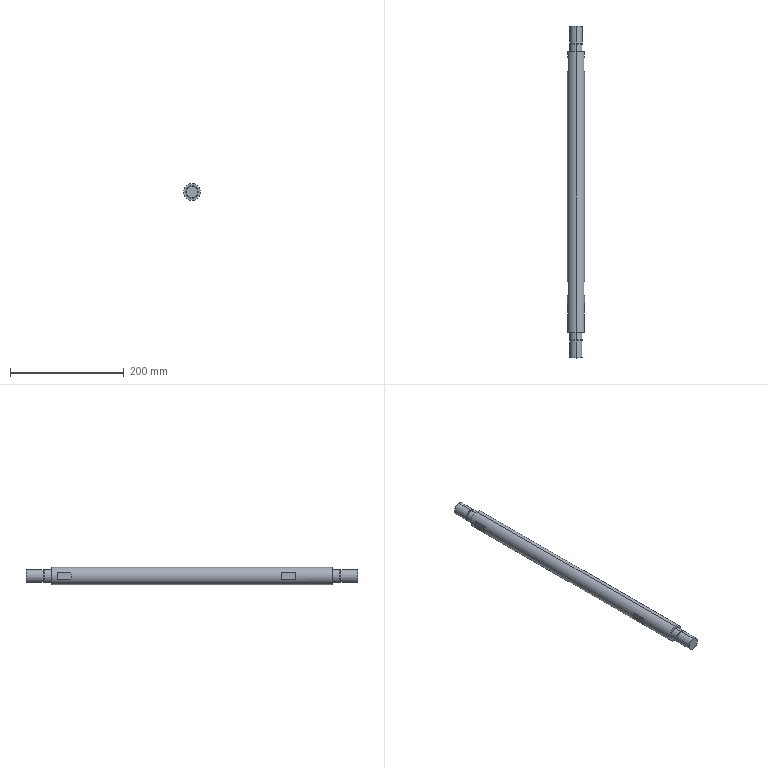Part | SolidWorks | features BaseBody 1 | 1 solid | 38 faces | box 30 x 585 x 30 mm | volume 382505 mm3 | plane 20 | cylinder 14 | cone 4 | commonest cylinder face diameters 22 x8 20 x4 30 x2
STEP:
#1=CARTESIAN_POINT('',(0.,30.,-11.));
#2=VERTEX_POINT('',#1);
#3=CARTESIAN_POINT('',(0.,30.,11.));
#4=VERTEX_POINT('',#3);
#5=CARTESIAN_POINT('',(0.,30.,0.));
#6=DIRECTION('',(0.,-1.,0.));
#7=DIRECTION('',(0.,0.,-1.));
#8=AXIS2_PLACEMENT_3D('',#5,#6,#7);
#9=CIRCLE('',#8,11.);
#10=EDGE_CURVE('',#2,#4,#9,.T.);
#11=ORIENTED_EDGE('',*,*,#10,.T.);
#12=CARTESIAN_POINT('',(0.,0.5,11.));
#13=VERTEX_POINT('',#12);
#14=CARTESIAN_POINT('',(0.,45.,11.));
#15=DIRECTION('',(0.,-1.,0.));
#16=VECTOR('',#15,1000.);
#17=LINE('',#14,#16);
#18=EDGE_CURVE('',#4,#13,#17,.T.);
#19=ORIENTED_EDGE('',*,*,#18,.T.);
#20=CARTESIAN_POINT('',(0.,0.5,-11.));
#21=VERTEX_POINT('',#20);
#22=CARTESIAN_POINT('',(0.,0.5,0.));
#23=DIRECTION('',(0.,1.,0.));
#24=DIRECTION('',(0.,0.,1.));
#25=AXIS2_PLACEMENT_3D('',#22,#23,#24);
#26=CIRCLE('',#25,11.);
#27=EDGE_CURVE('',#13,#21,#26,.T.);
#28=ORIENTED_EDGE('',*,*,#27,.T.);
#29=CARTESIAN_POINT('',(0.,45.,-11.));
#30=DIRECTION('',(0.,-1.,0.));
#31=VECTOR('',#30,1000.);
#32=LINE('',#29,#31);
#33=EDGE_CURVE('',#2,#21,#32,.T.);
#34=ORIENTED_EDGE('',*,*,#33,.F.);
#35=EDGE_LOOP('',(#11,#19,#28,#34));
#36=FACE_OUTER_BOUND('',#35,.T.);
#37=CARTESIAN_POINT('',(0.,45.,0.));
#38=DIRECTION('',(0.,-1.,0.));
#39=DIRECTION('',(0.,0.,-1.));
#40=AXIS2_PLACEMENT_3D('',#37,#38,#39);
#41=CYLINDRICAL_SURFACE('',#40,11.);
#42=ADVANCED_FACE('',(#36),#41,.T.);
#43=CARTESIAN_POINT('',(0.,0.,-10.5));
#44=VERTEX_POINT('',#43);
#45=CARTESIAN_POINT('',(0.,0.,10.5));
#46=VERTEX_POINT('',#45);
#47=CARTESIAN_POINT('',(0.,0.,0.));
#48=DIRECTION('',(0.,-1.,0.));
#49=DIRECTION('',(0.,0.,1.));
#50=AXIS2_PLACEMENT_3D('',#47,#48,#49);
#51=CIRCLE('',#50,10.5);
#52=EDGE_CURVE('',#44,#46,#51,.T.);
#53=ORIENTED_EDGE('',*,*,#52,.F.);
#54=CARTESIAN_POINT('',(0.,0.,-10.5));
#55=DIRECTION('',(0.,0.7071,-0.7071));
#56=VECTOR('',#55,1000.);
#57=LINE('',#54,#56);
#58=EDGE_CURVE('',#44,#21,#57,.T.);
#59=ORIENTED_EDGE('',*,*,#58,.T.);
#60=ORIENTED_EDGE('',*,*,#27,.F.);
#61=CARTESIAN_POINT('',(0.,0.,10.5));
#62=DIRECTION('',(0.,0.7071,0.7071));
#63=VECTOR('',#62,1000.);
#64=LINE('',#61,#63);
#65=EDGE_CURVE('',#46,#13,#64,.T.);
#66=ORIENTED_EDGE('',*,*,#65,.F.);
#67=EDGE_LOOP('',(#53,#59,#60,#66));
#68=FACE_OUTER_BOUND('',#67,.T.);
#69=CARTESIAN_POINT('',(0.,0.,0.));
#70=DIRECTION('',(0.,1.,0.));
#71=DIRECTION('',(0.,0.,1.));
#72=AXIS2_PLACEMENT_3D('',#69,#70,#71);
#73=CONICAL_SURFACE('',#72,10.5,0.7854);
#74=ADVANCED_FACE('',(#68),#73,.T.);
#75=CARTESIAN_POINT('',(0.,32.,-10.));
#76=VERTEX_POINT('',#75);
#77=CARTESIAN_POINT('',(0.,32.,10.));
#78=VERTEX_POINT('',#77);
#79=CARTESIAN_POINT('',(0.,32.,0.));
#80=DIRECTION('',(0.,-1.,0.));
#81=DIRECTION('',(0.,0.,-1.));
#82=AXIS2_PLACEMENT_3D('',#79,#80,#81);
#83=CIRCLE('',#82,10.);
#84=EDGE_CURVE('',#76,#78,#83,.T.);
#85=ORIENTED_EDGE('',*,*,#84,.T.);
#86=CARTESIAN_POINT('',(0.,30.,10.));
#87=VERTEX_POINT('',#86);
#88=CARTESIAN_POINT('',(0.,0.,10.));
#89=DIRECTION('',(0.,-1.,0.));
#90=VECTOR('',#89,1000.);
#91=LINE('',#88,#90);
#92=EDGE_CURVE('',#78,#87,#91,.T.);
#93=ORIENTED_EDGE('',*,*,#92,.T.);
#94=CARTESIAN_POINT('',(0.,30.,-10.));
#95=VERTEX_POINT('',#94);
#96=CARTESIAN_POINT('',(0.,30.,0.));
#97=DIRECTION('',(0.,-1.,0.));
#98=DIRECTION('',(0.,0.,-1.));
#99=AXIS2_PLACEMENT_3D('',#96,#97,#98);
#100=CIRCLE('',#99,10.);
#101=EDGE_CURVE('',#95,#87,#100,.T.);
#102=ORIENTED_EDGE('',*,*,#101,.F.);
#103=CARTESIAN_POINT('',(0.,0.,-10.));
#104=DIRECTION('',(0.,-1.,0.));
#105=VECTOR('',#104,1000.);
#106=LINE('',#103,#105);
#107=EDGE_CURVE('',#76,#95,#106,.T.);
#108=ORIENTED_EDGE('',*,*,#107,.F.);
#109=EDGE_LOOP('',(#85,#93,#102,#108));
#110=FACE_OUTER_BOUND('',#109,.T.);
#111=CARTESIAN_POINT('',(0.,0.,0.));
#112=DIRECTION('',(0.,-1.,0.));
#113=DIRECTION('',(0.,0.,-1.));
#114=AXIS2_PLACEMENT_3D('',#111,#112,#113);
#115=CYLINDRICAL_SURFACE('',#114,10.);
#116=ADVANCED_FACE('',(#110),#115,.T.);
#117=CARTESIAN_POINT('',(0.,45.,-11.));
#118=VERTEX_POINT('',#117);
#119=CARTESIAN_POINT('',(0.,45.,11.));
#120=VERTEX_POINT('',#119);
#121=CARTESIAN_POINT('',(0.,45.,0.));
#122=DIRECTION('',(0.,-1.,0.));
#123=DIRECTION('',(0.,0.,-1.));
#124=AXIS2_PLACEMENT_3D('',#121,#122,#123);
#125=CIRCLE('',#124,11.);
#126=EDGE_CURVE('',#118,#120,#125,.T.);
#127=ORIENTED_EDGE('',*,*,#126,.T.);
#128=CARTESIAN_POINT('',(0.,32.,11.));
#129=VERTEX_POINT('',#128);
#130=CARTESIAN_POINT('',(0.,45.,11.));
#131=DIRECTION('',(0.,-1.,0.));
#132=VECTOR('',#131,1000.);
#133=LINE('',#130,#132);
#134=EDGE_CURVE('',#120,#129,#133,.T.);
#135=ORIENTED_EDGE('',*,*,#134,.T.);
#136=CARTESIAN_POINT('',(0.,32.,-11.));
#137=VERTEX_POINT('',#136);
#138=CARTESIAN_POINT('',(0.,32.,0.));
#139=DIRECTION('',(0.,-1.,0.));
#140=DIRECTION('',(0.,0.,-1.));
#141=AXIS2_PLACEMENT_3D('',#138,#139,#140);
#142=CIRCLE('',#141,11.);
#143=EDGE_CURVE('',#137,#129,#142,.T.);
#144=ORIENTED_EDGE('',*,*,#143,.F.);
#145=CARTESIAN_POINT('',(0.,45.,-11.));
#146=DIRECTION('',(0.,-1.,0.));
#147=VECTOR('',#146,1000.);
#148=LINE('',#145,#147);
#149=EDGE_CURVE('',#118,#137,#148,.T.);
#150=ORIENTED_EDGE('',*,*,#149,.F.);
#151=EDGE_LOOP('',(#127,#135,#144,#150));
#152=FACE_OUTER_BOUND('',#151,.T.);
#153=CARTESIAN_POINT('',(0.,45.,0.));
#154=DIRECTION('',(0.,-1.,0.));
#155=DIRECTION('',(0.,0.,-1.));
#156=AXIS2_PLACEMENT_3D('',#153,#154,#155);
#157=CYLINDRICAL_SURFACE('',#156,11.);
#158=ADVANCED_FACE('',(#152),#157,.T.);
#159=CARTESIAN_POINT('',(13.5,505.,6.538));
#160=VERTEX_POINT('',#159);
#161=CARTESIAN_POINT('',(13.5,530.,6.538));
#162=VERTEX_POINT('',#161);
#163=CARTESIAN_POINT('',(13.5,585.,6.538));
#164=DIRECTION('',(0.,1.,0.));
#165=VECTOR('',#164,1000.);
#166=LINE('',#163,#165);
#167=EDGE_CURVE('',#160,#162,#166,.T.);
#168=ORIENTED_EDGE('',*,*,#167,.T.);
#169=CARTESIAN_POINT('',(13.5,530.,-6.538));
#170=VERTEX_POINT('',#169);
#171=CARTESIAN_POINT('',(0.,530.,0.));
#172=DIRECTION('',(0.,1.,0.));
#173=DIRECTION('',(0.,0.,1.));
#174=AXIS2_PLACEMENT_3D('',#171,#172,#173);
#175=CIRCLE('',#174,15.);
#176=EDGE_CURVE('',#162,#170,#175,.T.);
#177=ORIENTED_EDGE('',*,*,#176,.T.);
#178=CARTESIAN_POINT('',(13.5,505.,-6.538));
#179=VERTEX_POINT('',#178);
#180=CARTESIAN_POINT('',(13.5,585.,-6.538));
#181=DIRECTION('',(0.,-1.,0.));
#182=VECTOR('',#181,1000.);
#183=LINE('',#180,#182);
#184=EDGE_CURVE('',#170,#179,#183,.T.);
#185=ORIENTED_EDGE('',*,*,#184,.T.);
#186=CARTESIAN_POINT('',(0.,505.,0.));
#187=DIRECTION('',(0.,-1.,0.));
#188=DIRECTION('',(0.,0.,-1.));
#189=AXIS2_PLACEMENT_3D('',#186,#187,#188);
#190=CIRCLE('',#189,15.);
#191=EDGE_CURVE('',#179,#160,#190,.T.);
#192=ORIENTED_EDGE('',*,*,#191,.T.);
#193=EDGE_LOOP('',(#168,#177,#185,#192));
#194=FACE_BOUND('',#193,.T.);
#195=CARTESIAN_POINT('',(13.5,135.,-6.538));
#196=VERTEX_POINT('',#195);
#197=CARTESIAN_POINT('',(13.5,110.,-6.538));
#198=VERTEX_POINT('',#197);
#199=CARTESIAN_POINT('',(13.5,585.,-6.538));
#200=DIRECTION('',(0.,-1.,0.));
#201=VECTOR('',#200,1000.);
#202=LINE('',#199,#201);
#203=EDGE_CURVE('',#196,#198,#202,.T.);
#204=ORIENTED_EDGE('',*,*,#203,.T.);
#205=CARTESIAN_POINT('',(13.5,110.,6.538));
#206=VERTEX_POINT('',#205);
#207=CARTESIAN_POINT('',(0.,110.,0.));
#208=DIRECTION('',(0.,-1.,0.));
#209=DIRECTION('',(0.,0.,-1.));
#210=AXIS2_PLACEMENT_3D('',#207,#208,#209);
#211=CIRCLE('',#210,15.);
#212=EDGE_CURVE('',#198,#206,#211,.T.);
#213=ORIENTED_EDGE('',*,*,#212,.T.);
#214=CARTESIAN_POINT('',(13.5,135.,6.538));
#215=VERTEX_POINT('',#214);
#216=CARTESIAN_POINT('',(13.5,585.,6.538));
#217=DIRECTION('',(0.,1.,0.));
#218=VECTOR('',#217,1000.);
#219=LINE('',#216,#218);
#220=EDGE_CURVE('',#206,#215,#219,.T.);
#221=ORIENTED_EDGE('',*,*,#220,.T.);
#222=CARTESIAN_POINT('',(0.,135.,0.));
#223=DIRECTION('',(0.,1.,0.));
#224=DIRECTION('',(0.,0.,1.));
#225=AXIS2_PLACEMENT_3D('',#222,#223,#224);
#226=CIRCLE('',#225,15.);
#227=EDGE_CURVE('',#215,#196,#226,.T.);
#228=ORIENTED_EDGE('',*,*,#227,.T.);
#229=EDGE_LOOP('',(#204,#213,#221,#228));
#230=FACE_BOUND('',#229,.T.);
#231=CARTESIAN_POINT('',(0.,540.,15.));
#232=VERTEX_POINT('',#231);
#233=CARTESIAN_POINT('',(0.,540.,-15.));
#234=VERTEX_POINT('',#233);
#235=CARTESIAN_POINT('',(0.,540.,0.));
#236=DIRECTION('',(0.,1.,0.));
#237=DIRECTION('',(0.,0.,1.));
#238=AXIS2_PLACEMENT_3D('',#235,#236,#237);
#239=CIRCLE('',#238,15.);
#240=EDGE_CURVE('',#232,#234,#239,.T.);
#241=ORIENTED_EDGE('',*,*,#240,.F.);
#242=CARTESIAN_POINT('',(0.,45.,15.));
#243=VERTEX_POINT('',#242);
#244=CARTESIAN_POINT('',(0.,585.,15.));
#245=DIRECTION('',(0.,-1.,0.));
#246=VECTOR('',#245,1000.);
#247=LINE('',#244,#246);
#248=EDGE_CURVE('',#232,#243,#247,.T.);
#249=ORIENTED_EDGE('',*,*,#248,.T.);
#250=CARTESIAN_POINT('',(0.,45.,-15.));
#251=VERTEX_POINT('',#250);
#252=CARTESIAN_POINT('',(0.,45.,0.));
#253=DIRECTION('',(0.,-1.,0.));
#254=DIRECTION('',(0.,0.,-1.));
#255=AXIS2_PLACEMENT_3D('',#252,#253,#254);
#256=CIRCLE('',#255,15.);
#257=EDGE_CURVE('',#251,#243,#256,.T.);
#258=ORIENTED_EDGE('',*,*,#257,.F.);
#259=CARTESIAN_POINT('',(0.,585.,-15.));
#260=DIRECTION('',(0.,-1.,0.));
#261=VECTOR('',#260,1000.);
#262=LINE('',#259,#261);
#263=EDGE_CURVE('',#234,#251,#262,.T.);
#264=ORIENTED_EDGE('',*,*,#263,.F.);
#265=EDGE_LOOP('',(#241,#249,#258,#264));
#266=FACE_OUTER_BOUND('',#265,.T.);
#267=CARTESIAN_POINT('',(0.,585.,0.));
#268=DIRECTION('',(0.,-1.,0.));
#269=DIRECTION('',(0.,0.,-1.));
#270=AXIS2_PLACEMENT_3D('',#267,#268,#269);
#271=CYLINDRICAL_SURFACE('',#270,15.);
#272=ADVANCED_FACE('',(#194,#230,#266),#271,.T.);
#273=CARTESIAN_POINT('',(0.,540.,11.));
#274=VERTEX_POINT('',#273);
#275=CARTESIAN_POINT('',(0.,540.,-11.));
#276=VERTEX_POINT('',#275);
#277=CARTESIAN_POINT('',(0.,540.,0.));
#278=DIRECTION('',(0.,1.,0.));
#279=DIRECTION('',(0.,0.,1.));
#280=AXIS2_PLACEMENT_3D('',#277,#278,#279);
#281=CIRCLE('',#280,11.);
#282=EDGE_CURVE('',#274,#276,#281,.T.);
#283=ORIENTED_EDGE('',*,*,#282,.T.);
#284=CARTESIAN_POINT('',(0.,553.,-11.));
#285=VERTEX_POINT('',#284);
#286=CARTESIAN_POINT('',(0.,540.,-11.));
#287=DIRECTION('',(0.,1.,0.));
#288=VECTOR('',#287,1000.);
#289=LINE('',#286,#288);
#290=EDGE_CURVE('',#276,#285,#289,.T.);
#291=ORIENTED_EDGE('',*,*,#290,.T.);
#292=CARTESIAN_POINT('',(0.,553.,11.));
#293=VERTEX_POINT('',#292);
#294=CARTESIAN_POINT('',(0.,553.,0.));
#295=DIRECTION('',(0.,-1.,0.));
#296=DIRECTION('',(0.,0.,-1.));
#297=AXIS2_PLACEMENT_3D('',#294,#295,#296);
#298=CIRCLE('',#297,11.);
#299=EDGE_CURVE('',#285,#293,#298,.T.);
#300=ORIENTED_EDGE('',*,*,#299,.T.);
#301=CARTESIAN_POINT('',(0.,540.,11.));
#302=DIRECTION('',(0.,1.,0.));
#303=VECTOR('',#302,1000.);
#304=LINE('',#301,#303);
#305=EDGE_CURVE('',#274,#293,#304,.T.);
#306=ORIENTED_EDGE('',*,*,#305,.F.);
#307=EDGE_LOOP('',(#283,#291,#300,#306));
#308=FACE_OUTER_BOUND('',#307,.T.);
#309=CARTESIAN_POINT('',(0.,540.,0.));
#310=DIRECTION('',(0.,1.,0.));
#311=DIRECTION('',(0.,0.,1.));
#312=AXIS2_PLACEMENT_3D('',#309,#310,#311);
#313=CYLINDRICAL_SURFACE('',#312,11.);
#314=ADVANCED_FACE('',(#308),#313,.T.);
#315=CARTESIAN_POINT('',(0.,555.,-10.));
#316=VERTEX_POINT('',#315);
#317=CARTESIAN_POINT('',(0.,555.,10.));
#318=VERTEX_POINT('',#317);
#319=CARTESIAN_POINT('',(0.,555.,0.));
#320=DIRECTION('',(0.,-1.,0.));
#321=DIRECTION('',(0.,0.,-1.));
#322=AXIS2_PLACEMENT_3D('',#319,#320,#321);
#323=CIRCLE('',#322,10.);
#324=EDGE_CURVE('',#316,#318,#323,.T.);
#325=ORIENTED_EDGE('',*,*,#324,.T.);
#326=CARTESIAN_POINT('',(0.,553.,10.));
#327=VERTEX_POINT('',#326);
#328=CARTESIAN_POINT('',(0.,0.,10.));
#329=DIRECTION('',(0.,-1.,0.));
#330=VECTOR('',#329,1000.);
#331=LINE('',#328,#330);
#332=EDGE_CURVE('',#318,#327,#331,.T.);
#333=ORIENTED_EDGE('',*,*,#332,.T.);
#334=CARTESIAN_POINT('',(0.,553.,-10.));
#335=VERTEX_POINT('',#334);
#336=CARTESIAN_POINT('',(0.,553.,0.));
#337=DIRECTION('',(0.,-1.,0.));
#338=DIRECTION('',(0.,0.,-1.));
#339=AXIS2_PLACEMENT_3D('',#336,#337,#338);
#340=CIRCLE('',#339,10.);
#341=EDGE_CURVE('',#335,#327,#340,.T.);
#342=ORIENTED_EDGE('',*,*,#341,.F.);
#343=CARTESIAN_POINT('',(0.,0.,-10.));
#344=DIRECTION('',(0.,-1.,0.));
#345=VECTOR('',#344,1000.);
#346=LINE('',#343,#345);
#347=EDGE_CURVE('',#316,#335,#346,.T.);
#348=ORIENTED_EDGE('',*,*,#347,.F.);
#349=EDGE_LOOP('',(#325,#333,#342,#348));
#350=FACE_OUTER_BOUND('',#349,.T.);
#351=CARTESIAN_POINT('',(0.,0.,0.));
#352=DIRECTION('',(0.,-1.,0.));
#353=DIRECTION('',(0.,0.,-1.));
#354=AXIS2_PLACEMENT_3D('',#351,#352,#353);
#355=CYLINDRICAL_SURFACE('',#354,10.);
#356=ADVANCED_FACE('',(#350),#355,.T.);
#357=CARTESIAN_POINT('',(0.,585.,10.5));
#358=VERTEX_POINT('',#357);
#359=CARTESIAN_POINT('',(0.,585.,-10.5));
#360=VERTEX_POINT('',#359);
#361=CARTESIAN_POINT('',(0.,585.,0.));
#362=DIRECTION('',(0.,1.,0.));
#363=DIRECTION('',(0.,0.,1.));
#364=AXIS2_PLACEMENT_3D('',#361,#362,#363);
#365=CIRCLE('',#364,10.5);
#366=EDGE_CURVE('',#358,#360,#365,.T.);
#367=ORIENTED_EDGE('',*,*,#366,.F.);
#368=CARTESIAN_POINT('',(0.,584.5,11.));
#369=VERTEX_POINT('',#368);
#370=CARTESIAN_POINT('',(0.,585.,10.5));
#371=DIRECTION('',(0.,-0.7071,0.7071));
#372=VECTOR('',#371,1000.);
#373=LINE('',#370,#372);
#374=EDGE_CURVE('',#358,#369,#373,.T.);
#375=ORIENTED_EDGE('',*,*,#374,.T.);
#376=CARTESIAN_POINT('',(0.,584.5,-11.));
#377=VERTEX_POINT('',#376);
#378=CARTESIAN_POINT('',(0.,584.5,0.));
#379=DIRECTION('',(0.,-1.,0.));
#380=DIRECTION('',(0.,0.,1.));
#381=AXIS2_PLACEMENT_3D('',#378,#379,#380);
#382=CIRCLE('',#381,11.);
#383=EDGE_CURVE('',#377,#369,#382,.T.);
#384=ORIENTED_EDGE('',*,*,#383,.F.);
#385=CARTESIAN_POINT('',(0.,585.,-10.5));
#386=DIRECTION('',(0.,-0.7071,-0.7071));
#387=VECTOR('',#386,1000.);
#388=LINE('',#385,#387);
#389=EDGE_CURVE('',#360,#377,#388,.T.);
#390=ORIENTED_EDGE('',*,*,#389,.F.);
#391=EDGE_LOOP('',(#367,#375,#384,#390));
#392=FACE_OUTER_BOUND('',#391,.T.);
#393=CARTESIAN_POINT('',(0.,585.,0.));
#394=DIRECTION('',(0.,-1.,0.));
#395=DIRECTION('',(0.,0.,-1.));
#396=AXIS2_PLACEMENT_3D('',#393,#394,#395);
#397=CONICAL_SURFACE('',#396,10.5,0.7854);
#398=ADVANCED_FACE('',(#392),#397,.T.);
#399=CARTESIAN_POINT('',(0.,555.,-11.));
#400=VERTEX_POINT('',#399);
#401=CARTESIAN_POINT('',(0.,555.,11.));
#402=VERTEX_POINT('',#401);
#403=CARTESIAN_POINT('',(0.,555.,0.));
#404=DIRECTION('',(0.,-1.,0.));
#405=DIRECTION('',(0.,0.,-1.));
#406=AXIS2_PLACEMENT_3D('',#403,#404,#405);
#407=CIRCLE('',#406,11.);
#408=EDGE_CURVE('',#400,#402,#407,.T.);
#409=ORIENTED_EDGE('',*,*,#408,.F.);
#410=CARTESIAN_POINT('',(0.,540.,-11.));
#411=DIRECTION('',(0.,1.,0.));
#412=VECTOR('',#411,1000.);
#413=LINE('',#410,#412);
#414=EDGE_CURVE('',#400,#377,#413,.T.);
#415=ORIENTED_EDGE('',*,*,#414,.T.);
#416=ORIENTED_EDGE('',*,*,#383,.T.);
#417=CARTESIAN_POINT('',(0.,540.,11.));
#418=DIRECTION('',(0.,1.,0.));
#419=VECTOR('',#418,1000.);
#420=LINE('',#417,#419);
#421=EDGE_CURVE('',#402,#369,#420,.T.);
#422=ORIENTED_EDGE('',*,*,#421,.F.);
#423=EDGE_LOOP('',(#409,#415,#416,#422));
#424=FACE_OUTER_BOUND('',#423,.T.);
#425=CARTESIAN_POINT('',(0.,540.,0.));
#426=DIRECTION('',(0.,1.,0.));
#427=DIRECTION('',(0.,0.,1.));
#428=AXIS2_PLACEMENT_3D('',#425,#426,#427);
#429=CYLINDRICAL_SURFACE('',#428,11.);
#430=ADVANCED_FACE('',(#424),#429,.T.);
#431=CARTESIAN_POINT('',(-13.5,505.,-6.538));
#432=VERTEX_POINT('',#431);
#433=CARTESIAN_POINT('',(-13.5,505.,6.538));
#434=VERTEX_POINT('',#433);
#435=CARTESIAN_POINT('',(-13.5,505.,-100.));
#436=DIRECTION('',(0.,0.,1.));
#437=VECTOR('',#436,1000.);
#438=LINE('',#435,#437);
#439=EDGE_CURVE('',#432,#434,#438,.T.);
#440=ORIENTED_EDGE('',*,*,#439,.F.);
#441=CARTESIAN_POINT('',(0.,505.,0.));
#442=DIRECTION('',(0.,-1.,0.));
#443=DIRECTION('',(0.,0.,-1.));
#444=AXIS2_PLACEMENT_3D('',#441,#442,#443);
#445=CIRCLE('',#444,15.);
#446=EDGE_CURVE('',#434,#432,#445,.T.);
#447=ORIENTED_EDGE('',*,*,#446,.F.);
#448=EDGE_LOOP('',(#440,#447));
#449=FACE_OUTER_BOUND('',#448,.T.);
#450=CARTESIAN_POINT('',(-13.5,505.,-100.));
#451=DIRECTION('',(0.,-1.,0.));
#452=DIRECTION('',(0.,0.,-1.));
#453=AXIS2_PLACEMENT_3D('',#450,#451,#452);
#454=PLANE('',#453);
#455=ADVANCED_FACE('',(#449),#454,.F.);
#456=CARTESIAN_POINT('',(-13.5,530.,-6.538));
#457=VERTEX_POINT('',#456);
#458=CARTESIAN_POINT('',(-13.5,530.,6.538));
#459=VERTEX_POINT('',#458);
#460=CARTESIAN_POINT('',(-13.5,530.,-100.));
#461=DIRECTION('',(0.,0.,1.));
#462=VECTOR('',#461,1000.);
#463=LINE('',#460,#462);
#464=EDGE_CURVE('',#457,#459,#463,.T.);
#465=ORIENTED_EDGE('',*,*,#464,.F.);
#466=CARTESIAN_POINT('',(-13.5,585.,-6.538));
#467=DIRECTION('',(0.,1.,0.));
#468=VECTOR('',#467,1000.);
#469=LINE('',#466,#468);
#470=EDGE_CURVE('',#432,#457,#469,.T.);
#471=ORIENTED_EDGE('',*,*,#470,.F.);
#472=ORIENTED_EDGE('',*,*,#439,.T.);
#473=CARTESIAN_POINT('',(-13.5,585.,6.538));
#474=DIRECTION('',(0.,-1.,0.));
#475=VECTOR('',#474,1000.);
#476=LINE('',#473,#475);
#477=EDGE_CURVE('',#459,#434,#476,.T.);
#478=ORIENTED_EDGE('',*,*,#477,.F.);
#479=EDGE_LOOP('',(#465,#471,#472,#478));
#480=FACE_OUTER_BOUND('',#479,.T.);
#481=CARTESIAN_POINT('',(-13.5,530.,-100.));
#482=DIRECTION('',(1.,0.,0.));
#483=DIRECTION('',(0.,-1.,0.));
#484=AXIS2_PLACEMENT_3D('',#481,#482,#483);
#485=PLANE('',#484);
#486=ADVANCED_FACE('',(#480),#485,.F.);
#487=ORIENTED_EDGE('',*,*,#464,.T.);
#488=CARTESIAN_POINT('',(0.,530.,0.));
#489=DIRECTION('',(0.,1.,0.));
#490=DIRECTION('',(0.,0.,1.));
#491=AXIS2_PLACEMENT_3D('',#488,#489,#490);
#492=CIRCLE('',#491,15.);
#493=EDGE_CURVE('',#457,#459,#492,.T.);
#494=ORIENTED_EDGE('',*,*,#493,.F.);
#495=EDGE_LOOP('',(#487,#494));
#496=FACE_OUTER_BOUND('',#495,.T.);
#497=CARTESIAN_POINT('',(-13.5,530.,-100.));
#498=DIRECTION('',(0.,1.,0.));
#499=DIRECTION('',(1.,0.,0.));
#500=AXIS2_PLACEMENT_3D('',#497,#498,#499);
#501=PLANE('',#500);
#502=ADVANCED_FACE('',(#496),#501,.F.);
#503=CARTESIAN_POINT('',(13.5,135.,-100.));
#504=DIRECTION('',(0.,0.,1.));
#505=VECTOR('',#504,1000.);
#506=LINE('',#503,#505);
#507=EDGE_CURVE('',#196,#215,#506,.T.);
#508=ORIENTED_EDGE('',*,*,#507,.F.);
#509=ORIENTED_EDGE('',*,*,#227,.F.);
#510=EDGE_LOOP('',(#508,#509));
#511=FACE_OUTER_BOUND('',#510,.T.);
#512=CARTESIAN_POINT('',(16.5,135.,-100.));
#513=DIRECTION('',(0.,1.,0.));
#514=DIRECTION('',(1.,0.,0.));
#515=AXIS2_PLACEMENT_3D('',#512,#513,#514);
#516=PLANE('',#515);
#517=ADVANCED_FACE('',(#511),#516,.F.);
#518=ORIENTED_EDGE('',*,*,#507,.T.);
#519=ORIENTED_EDGE('',*,*,#220,.F.);
#520=CARTESIAN_POINT('',(13.5,110.,-100.));
#521=DIRECTION('',(0.,0.,1.));
#522=VECTOR('',#521,1000.);
#523=LINE('',#520,#522);
#524=EDGE_CURVE('',#198,#206,#523,.T.);
#525=ORIENTED_EDGE('',*,*,#524,.F.);
#526=ORIENTED_EDGE('',*,*,#203,.F.);
#527=EDGE_LOOP('',(#518,#519,#525,#526));
#528=FACE_OUTER_BOUND('',#527,.T.);
#529=CARTESIAN_POINT('',(13.5,110.,-100.));
#530=DIRECTION('',(-1.,0.,0.));
#531=DIRECTION('',(0.,0.,1.));
#532=AXIS2_PLACEMENT_3D('',#529,#530,#531);
#533=PLANE('',#532);
#534=ADVANCED_FACE('',(#528),#533,.F.);
#535=ORIENTED_EDGE('',*,*,#524,.T.);
#536=ORIENTED_EDGE('',*,*,#212,.F.);
#537=EDGE_LOOP('',(#535,#536));
#538=FACE_OUTER_BOUND('',#537,.T.);
#539=CARTESIAN_POINT('',(16.5,110.,-100.));
#540=DIRECTION('',(0.,-1.,0.));
#541=DIRECTION('',(0.,0.,-1.));
#542=AXIS2_PLACEMENT_3D('',#539,#540,#541);
#543=PLANE('',#542);
#544=ADVANCED_FACE('',(#538),#543,.F.);
#545=CARTESIAN_POINT('',(-13.5,110.,-6.538));
#546=VERTEX_POINT('',#545);
#547=CARTESIAN_POINT('',(-13.5,110.,6.538));
#548=VERTEX_POINT('',#547);
#549=CARTESIAN_POINT('',(-13.5,110.,-100.));
#550=DIRECTION('',(0.,0.,1.));
#551=VECTOR('',#550,1000.);
#552=LINE('',#549,#551);
#553=EDGE_CURVE('',#546,#548,#552,.T.);
#554=ORIENTED_EDGE('',*,*,#553,.F.);
#555=CARTESIAN_POINT('',(0.,110.,0.));
#556=DIRECTION('',(0.,-1.,0.));
#557=DIRECTION('',(0.,0.,-1.));
#558=AXIS2_PLACEMENT_3D('',#555,#556,#557);
#559=CIRCLE('',#558,15.);
#560=EDGE_CURVE('',#548,#546,#559,.T.);
#561=ORIENTED_EDGE('',*,*,#560,.F.);
#562=EDGE_LOOP('',(#554,#561));
#563=FACE_OUTER_BOUND('',#562,.T.);
#564=CARTESIAN_POINT('',(-16.5,110.,-100.));
#565=DIRECTION('',(0.,-1.,0.));
#566=DIRECTION('',(0.,0.,-1.));
#567=AXIS2_PLACEMENT_3D('',#564,#565,#566);
#568=PLANE('',#567);
#569=ADVANCED_FACE('',(#563),#568,.F.);
#570=CARTESIAN_POINT('',(-13.5,135.,-6.538));
#571=VERTEX_POINT('',#570);
#572=CARTESIAN_POINT('',(-13.5,135.,6.538));
#573=VERTEX_POINT('',#572);
#574=CARTESIAN_POINT('',(-13.5,135.,-100.));
#575=DIRECTION('',(0.,0.,1.));
#576=VECTOR('',#575,1000.);
#577=LINE('',#574,#576);
#578=EDGE_CURVE('',#571,#573,#577,.T.);
#579=ORIENTED_EDGE('',*,*,#578,.F.);
#580=CARTESIAN_POINT('',(-13.5,585.,-6.538));
#581=DIRECTION('',(0.,1.,0.));
#582=VECTOR('',#581,1000.);
#583=LINE('',#580,#582);
#584=EDGE_CURVE('',#546,#571,#583,.T.);
#585=ORIENTED_EDGE('',*,*,#584,.F.);
#586=ORIENTED_EDGE('',*,*,#553,.T.);
#587=CARTESIAN_POINT('',(-13.5,585.,6.538));
#588=DIRECTION('',(0.,-1.,0.));
#589=VECTOR('',#588,1000.);
#590=LINE('',#587,#589);
#591=EDGE_CURVE('',#573,#548,#590,.T.);
#592=ORIENTED_EDGE('',*,*,#591,.F.);
#593=EDGE_LOOP('',(#579,#585,#586,#592));
#594=FACE_OUTER_BOUND('',#593,.T.);
#595=CARTESIAN_POINT('',(-13.5,110.,-100.));
#596=DIRECTION('',(1.,0.,0.));
#597=DIRECTION('',(0.,1.,0.));
#598=AXIS2_PLACEMENT_3D('',#595,#596,#597);
#599=PLANE('',#598);
#600=ADVANCED_FACE('',(#594),#599,.F.);
#601=ORIENTED_EDGE('',*,*,#578,.T.);
#602=CARTESIAN_POINT('',(0.,135.,0.));
#603=DIRECTION('',(0.,1.,0.));
#604=DIRECTION('',(0.,0.,1.));
#605=AXIS2_PLACEMENT_3D('',#602,#603,#604);
#606=CIRCLE('',#605,15.);
#607=EDGE_CURVE('',#571,#573,#606,.T.);
#608=ORIENTED_EDGE('',*,*,#607,.F.);
#609=EDGE_LOOP('',(#601,#608));
#610=FACE_OUTER_BOUND('',#609,.T.);
#611=CARTESIAN_POINT('',(-16.5,135.,-100.));
#612=DIRECTION('',(0.,1.,0.));
#613=DIRECTION('',(1.,0.,0.));
#614=AXIS2_PLACEMENT_3D('',#611,#612,#613);
#615=PLANE('',#614);
#616=ADVANCED_FACE('',(#610),#615,.F.);
#617=CARTESIAN_POINT('',(13.5,505.,-100.));
#618=DIRECTION('',(0.,0.,1.));
#619=VECTOR('',#618,1000.);
#620=LINE('',#617,#619);
#621=EDGE_CURVE('',#179,#160,#620,.T.);
#622=ORIENTED_EDGE('',*,*,#621,.T.);
#623=ORIENTED_EDGE('',*,*,#191,.F.);
#624=EDGE_LOOP('',(#622,#623));
#625=FACE_OUTER_BOUND('',#624,.T.);
#626=CARTESIAN_POINT('',(13.5,505.,-100.));
#627=DIRECTION('',(0.,-1.,0.));
#628=DIRECTION('',(0.,0.,-1.));
#629=AXIS2_PLACEMENT_3D('',#626,#627,#628);
#630=PLANE('',#629);
#631=ADVANCED_FACE('',(#625),#630,.F.);
#632=CARTESIAN_POINT('',(13.5,530.,-100.));
#633=DIRECTION('',(0.,0.,1.));
#634=VECTOR('',#633,1000.);
#635=LINE('',#632,#634);
#636=EDGE_CURVE('',#170,#162,#635,.T.);
#637=ORIENTED_EDGE('',*,*,#636,.F.);
#638=ORIENTED_EDGE('',*,*,#176,.F.);
#639=EDGE_LOOP('',(#637,#638));
#640=FACE_OUTER_BOUND('',#639,.T.);
#641=CARTESIAN_POINT('',(13.5,530.,-100.));
#642=DIRECTION('',(0.,1.,0.));
#643=DIRECTION('',(1.,0.,0.));
#644=AXIS2_PLACEMENT_3D('',#641,#642,#643);
#645=PLANE('',#644);
#646=ADVANCED_FACE('',(#640),#645,.F.);
#647=ORIENTED_EDGE('',*,*,#636,.T.);
#648=ORIENTED_EDGE('',*,*,#167,.F.);
#649=ORIENTED_EDGE('',*,*,#621,.F.);
#650=ORIENTED_EDGE('',*,*,#184,.F.);
#651=EDGE_LOOP('',(#647,#648,#649,#650));
#652=FACE_OUTER_BOUND('',#651,.T.);
#653=CARTESIAN_POINT('',(13.5,530.,-100.));
#654=DIRECTION('',(-1.,0.,0.));
#655=DIRECTION('',(0.,1.,0.));
#656=AXIS2_PLACEMENT_3D('',#653,#654,#655);
#657=PLANE('',#656);
#658=ADVANCED_FACE('',(#652),#657,.F.);
#659=CARTESIAN_POINT('',(0.,0.,0.));
#660=DIRECTION('',(0.,-1.,0.));
#661=DIRECTION('',(0.,0.,1.));
#662=AXIS2_PLACEMENT_3D('',#659,#660,#661);
#663=CIRCLE('',#662,10.5);
#664=EDGE_CURVE('',#46,#44,#663,.T.);
#665=ORIENTED_EDGE('',*,*,#664,.T.);
#666=ORIENTED_EDGE('',*,*,#52,.T.);
#667=EDGE_LOOP('',(#665,#666));
#668=FACE_OUTER_BOUND('',#667,.T.);
#669=CARTESIAN_POINT('',(0.,0.,0.));
#670=DIRECTION('',(0.,1.,0.));
#671=DIRECTION('',(1.,0.,0.));
#672=AXIS2_PLACEMENT_3D('',#669,#670,#671);
#673=PLANE('',#672);
#674=ADVANCED_FACE('',(#668),#673,.F.);
#675=ORIENTED_EDGE('',*,*,#101,.T.);
#676=CARTESIAN_POINT('',(0.,30.,0.));
#677=DIRECTION('',(0.,-1.,0.));
#678=DIRECTION('',(0.,0.,-1.));
#679=AXIS2_PLACEMENT_3D('',#676,#677,#678);
#680=CIRCLE('',#679,10.);
#681=EDGE_CURVE('',#87,#95,#680,.T.);
#682=ORIENTED_EDGE('',*,*,#681,.T.);
#683=EDGE_LOOP('',(#675,#682));
#684=FACE_BOUND('',#683,.T.);
#685=ORIENTED_EDGE('',*,*,#10,.F.);
#686=CARTESIAN_POINT('',(0.,30.,0.));
#687=DIRECTION('',(0.,-1.,0.));
#688=DIRECTION('',(0.,0.,-1.));
#689=AXIS2_PLACEMENT_3D('',#686,#687,#688);
#690=CIRCLE('',#689,11.);
#691=EDGE_CURVE('',#4,#2,#690,.T.);
#692=ORIENTED_EDGE('',*,*,#691,.F.);
#693=EDGE_LOOP('',(#685,#692));
#694=FACE_OUTER_BOUND('',#693,.T.);
#695=CARTESIAN_POINT('',(10.,30.,0.));
#696=DIRECTION('',(0.,-1.,0.));
#697=DIRECTION('',(0.,0.,-1.));
#698=AXIS2_PLACEMENT_3D('',#695,#696,#697);
#699=PLANE('',#698);
#700=ADVANCED_FACE('',(#684,#694),#699,.F.);
#701=ORIENTED_EDGE('',*,*,#84,.F.);
#702=CARTESIAN_POINT('',(0.,32.,0.));
#703=DIRECTION('',(0.,-1.,0.));
#704=DIRECTION('',(0.,0.,-1.));
#705=AXIS2_PLACEMENT_3D('',#702,#703,#704);
#706=CIRCLE('',#705,10.);
#707=EDGE_CURVE('',#78,#76,#706,.T.);
#708=ORIENTED_EDGE('',*,*,#707,.F.);
#709=EDGE_LOOP('',(#701,#708));
#710=FACE_BOUND('',#709,.T.);
#711=ORIENTED_EDGE('',*,*,#143,.T.);
#712=CARTESIAN_POINT('',(0.,32.,0.));
#713=DIRECTION('',(0.,-1.,0.));
#714=DIRECTION('',(0.,0.,-1.));
#715=AXIS2_PLACEMENT_3D('',#712,#713,#714);
#716=CIRCLE('',#715,11.);
#717=EDGE_CURVE('',#129,#137,#716,.T.);
#718=ORIENTED_EDGE('',*,*,#717,.T.);
#719=EDGE_LOOP('',(#711,#718));
#720=FACE_OUTER_BOUND('',#719,.T.);
#721=CARTESIAN_POINT('',(10.,32.,0.));
#722=DIRECTION('',(0.,1.,0.));
#723=DIRECTION('',(1.,0.,0.));
#724=AXIS2_PLACEMENT_3D('',#721,#722,#723);
#725=PLANE('',#724);
#726=ADVANCED_FACE('',(#710,#720),#725,.F.);
#727=ORIENTED_EDGE('',*,*,#126,.F.);
#728=CARTESIAN_POINT('',(0.,45.,0.));
#729=DIRECTION('',(0.,-1.,0.));
#730=DIRECTION('',(0.,0.,-1.));
#731=AXIS2_PLACEMENT_3D('',#728,#729,#730);
#732=CIRCLE('',#731,11.);
#733=EDGE_CURVE('',#120,#118,#732,.T.);
#734=ORIENTED_EDGE('',*,*,#733,.F.);
#735=EDGE_LOOP('',(#727,#734));
#736=FACE_BOUND('',#735,.T.);
#737=ORIENTED_EDGE('',*,*,#257,.T.);
#738=CARTESIAN_POINT('',(0.,45.,0.));
#739=DIRECTION('',(0.,-1.,0.));
#740=DIRECTION('',(0.,0.,-1.));
#741=AXIS2_PLACEMENT_3D('',#738,#739,#740);
#742=CIRCLE('',#741,15.);
#743=EDGE_CURVE('',#243,#251,#742,.T.);
#744=ORIENTED_EDGE('',*,*,#743,.T.);
#745=EDGE_LOOP('',(#737,#744));
#746=FACE_OUTER_BOUND('',#745,.T.);
#747=CARTESIAN_POINT('',(0.,45.,0.));
#748=DIRECTION('',(0.,-1.,0.));
#749=DIRECTION('',(0.,0.,-1.));
#750=AXIS2_PLACEMENT_3D('',#747,#748,#749);
#751=PLANE('',#750);
#752=ADVANCED_FACE('',(#736,#746),#751,.T.);
#753=ORIENTED_EDGE('',*,*,#282,.F.);
#754=CARTESIAN_POINT('',(0.,540.,0.));
#755=DIRECTION('',(0.,1.,0.));
#756=DIRECTION('',(0.,0.,1.));
#757=AXIS2_PLACEMENT_3D('',#754,#755,#756);
#758=CIRCLE('',#757,11.);
#759=EDGE_CURVE('',#276,#274,#758,.T.);
#760=ORIENTED_EDGE('',*,*,#759,.F.);
#761=EDGE_LOOP('',(#753,#760));
#762=FACE_BOUND('',#761,.T.);
#763=CARTESIAN_POINT('',(0.,540.,0.));
#764=DIRECTION('',(0.,1.,0.));
#765=DIRECTION('',(0.,0.,1.));
#766=AXIS2_PLACEMENT_3D('',#763,#764,#765);
#767=CIRCLE('',#766,15.);
#768=EDGE_CURVE('',#234,#232,#767,.T.);
#769=ORIENTED_EDGE('',*,*,#768,.T.);
#770=ORIENTED_EDGE('',*,*,#240,.T.);
#771=EDGE_LOOP('',(#769,#770));
#772=FACE_OUTER_BOUND('',#771,.T.);
#773=CARTESIAN_POINT('',(0.,540.,0.));
#774=DIRECTION('',(0.,1.,0.));
#775=DIRECTION('',(1.,0.,0.));
#776=AXIS2_PLACEMENT_3D('',#773,#774,#775);
#777=PLANE('',#776);
#778=ADVANCED_FACE('',(#762,#772),#777,.T.);
#779=ORIENTED_EDGE('',*,*,#341,.T.);
#780=CARTESIAN_POINT('',(0.,553.,0.));
#781=DIRECTION('',(0.,-1.,0.));
#782=DIRECTION('',(0.,0.,-1.));
#783=AXIS2_PLACEMENT_3D('',#780,#781,#782);
#784=CIRCLE('',#783,10.);
#785=EDGE_CURVE('',#327,#335,#784,.T.);
#786=ORIENTED_EDGE('',*,*,#785,.T.);
#787=EDGE_LOOP('',(#779,#786));
#788=FACE_BOUND('',#787,.T.);
#789=CARTESIAN_POINT('',(0.,553.,0.));
#790=DIRECTION('',(0.,-1.,0.));
#791=DIRECTION('',(0.,0.,-1.));
#792=AXIS2_PLACEMENT_3D('',#789,#790,#791);
#793=CIRCLE('',#792,11.);
#794=EDGE_CURVE('',#293,#285,#793,.T.);
#795=ORIENTED_EDGE('',*,*,#794,.F.);
#796=ORIENTED_EDGE('',*,*,#299,.F.);
#797=EDGE_LOOP('',(#795,#796));
#798=FACE_OUTER_BOUND('',#797,.T.);
#799=CARTESIAN_POINT('',(11.,553.,0.));
#800=DIRECTION('',(0.,-1.,0.));
#801=DIRECTION('',(0.,0.,-1.));
#802=AXIS2_PLACEMENT_3D('',#799,#800,#801);
#803=PLANE('',#802);
#804=ADVANCED_FACE('',(#788,#798),#803,.F.);
#805=ORIENTED_EDGE('',*,*,#324,.F.);
#806=CARTESIAN_POINT('',(0.,555.,0.));
#807=DIRECTION('',(0.,-1.,0.));
#808=DIRECTION('',(0.,0.,-1.));
#809=AXIS2_PLACEMENT_3D('',#806,#807,#808);
#810=CIRCLE('',#809,10.);
#811=EDGE_CURVE('',#318,#316,#810,.T.);
#812=ORIENTED_EDGE('',*,*,#811,.F.);
#813=EDGE_LOOP('',(#805,#812));
#814=FACE_BOUND('',#813,.T.);
#815=CARTESIAN_POINT('',(0.,555.,0.));
#816=DIRECTION('',(0.,-1.,0.));
#817=DIRECTION('',(0.,0.,-1.));
#818=AXIS2_PLACEMENT_3D('',#815,#816,#817);
#819=CIRCLE('',#818,11.);
#820=EDGE_CURVE('',#402,#400,#819,.T.);
#821=ORIENTED_EDGE('',*,*,#820,.T.);
#822=ORIENTED_EDGE('',*,*,#408,.T.);
#823=EDGE_LOOP('',(#821,#822));
#824=FACE_OUTER_BOUND('',#823,.T.);
#825=CARTESIAN_POINT('',(11.,555.,0.));
#826=DIRECTION('',(0.,1.,0.));
#827=DIRECTION('',(1.,0.,0.));
#828=AXIS2_PLACEMENT_3D('',#825,#826,#827);
#829=PLANE('',#828);
#830=ADVANCED_FACE('',(#814,#824),#829,.F.);
#831=CARTESIAN_POINT('',(0.,585.,0.));
#832=DIRECTION('',(0.,1.,0.));
#833=DIRECTION('',(0.,0.,1.));
#834=AXIS2_PLACEMENT_3D('',#831,#832,#833);
#835=CIRCLE('',#834,10.5);
#836=EDGE_CURVE('',#360,#358,#835,.T.);
#837=ORIENTED_EDGE('',*,*,#836,.T.);
#838=ORIENTED_EDGE('',*,*,#366,.T.);
#839=EDGE_LOOP('',(#837,#838));
#840=FACE_OUTER_BOUND('',#839,.T.);
#841=CARTESIAN_POINT('',(0.,585.,0.));
#842=DIRECTION('',(0.,1.,0.));
#843=DIRECTION('',(1.,0.,0.));
#844=AXIS2_PLACEMENT_3D('',#841,#842,#843);
#845=PLANE('',#844);
#846=ADVANCED_FACE('',(#840),#845,.T.);
#847=ORIENTED_EDGE('',*,*,#414,.F.);
#848=ORIENTED_EDGE('',*,*,#820,.F.);
#849=ORIENTED_EDGE('',*,*,#421,.T.);
#850=CARTESIAN_POINT('',(0.,584.5,0.));
#851=DIRECTION('',(0.,-1.,0.));
#852=DIRECTION('',(0.,0.,1.));
#853=AXIS2_PLACEMENT_3D('',#850,#851,#852);
#854=CIRCLE('',#853,11.);
#855=EDGE_CURVE('',#369,#377,#854,.T.);
#856=ORIENTED_EDGE('',*,*,#855,.T.);
#857=EDGE_LOOP('',(#847,#848,#849,#856));
#858=FACE_OUTER_BOUND('',#857,.T.);
#859=CARTESIAN_POINT('',(0.,540.,0.));
#860=DIRECTION('',(0.,1.,0.));
#861=DIRECTION('',(0.,0.,1.));
#862=AXIS2_PLACEMENT_3D('',#859,#860,#861);
#863=CYLINDRICAL_SURFACE('',#862,11.);
#864=ADVANCED_FACE('',(#858),#863,.T.);
#865=ORIENTED_EDGE('',*,*,#374,.F.);
#866=ORIENTED_EDGE('',*,*,#836,.F.);
#867=ORIENTED_EDGE('',*,*,#389,.T.);
#868=ORIENTED_EDGE('',*,*,#855,.F.);
#869=EDGE_LOOP('',(#865,#866,#867,#868));
#870=FACE_OUTER_BOUND('',#869,.T.);
#871=CARTESIAN_POINT('',(0.,585.,0.));
#872=DIRECTION('',(0.,-1.,0.));
#873=DIRECTION('',(0.,0.,-1.));
#874=AXIS2_PLACEMENT_3D('',#871,#872,#873);
#875=CONICAL_SURFACE('',#874,10.5,0.7854);
#876=ADVANCED_FACE('',(#870),#875,.T.);
#877=ORIENTED_EDGE('',*,*,#332,.F.);
#878=ORIENTED_EDGE('',*,*,#811,.T.);
#879=ORIENTED_EDGE('',*,*,#347,.T.);
#880=ORIENTED_EDGE('',*,*,#785,.F.);
#881=EDGE_LOOP('',(#877,#878,#879,#880));
#882=FACE_OUTER_BOUND('',#881,.T.);
#883=CARTESIAN_POINT('',(0.,0.,0.));
#884=DIRECTION('',(0.,-1.,0.));
#885=DIRECTION('',(0.,0.,-1.));
#886=AXIS2_PLACEMENT_3D('',#883,#884,#885);
#887=CYLINDRICAL_SURFACE('',#886,10.);
#888=ADVANCED_FACE('',(#882),#887,.T.);
#889=ORIENTED_EDGE('',*,*,#290,.F.);
#890=ORIENTED_EDGE('',*,*,#759,.T.);
#891=ORIENTED_EDGE('',*,*,#305,.T.);
#892=ORIENTED_EDGE('',*,*,#794,.T.);
#893=EDGE_LOOP('',(#889,#890,#891,#892));
#894=FACE_OUTER_BOUND('',#893,.T.);
#895=CARTESIAN_POINT('',(0.,540.,0.));
#896=DIRECTION('',(0.,1.,0.));
#897=DIRECTION('',(0.,0.,1.));
#898=AXIS2_PLACEMENT_3D('',#895,#896,#897);
#899=CYLINDRICAL_SURFACE('',#898,11.);
#900=ADVANCED_FACE('',(#894),#899,.T.);
#901=ORIENTED_EDGE('',*,*,#248,.F.);
#902=ORIENTED_EDGE('',*,*,#768,.F.);
#903=ORIENTED_EDGE('',*,*,#263,.T.);
#904=ORIENTED_EDGE('',*,*,#743,.F.);
#905=EDGE_LOOP('',(#901,#902,#903,#904));
#906=FACE_OUTER_BOUND('',#905,.T.);
#907=ORIENTED_EDGE('',*,*,#584,.T.);
#908=ORIENTED_EDGE('',*,*,#607,.T.);
#909=ORIENTED_EDGE('',*,*,#591,.T.);
#910=ORIENTED_EDGE('',*,*,#560,.T.);
#911=EDGE_LOOP('',(#907,#908,#909,#910));
#912=FACE_BOUND('',#911,.T.);
#913=ORIENTED_EDGE('',*,*,#470,.T.);
#914=ORIENTED_EDGE('',*,*,#493,.T.);
#915=ORIENTED_EDGE('',*,*,#477,.T.);
#916=ORIENTED_EDGE('',*,*,#446,.T.);
#917=EDGE_LOOP('',(#913,#914,#915,#916));
#918=FACE_BOUND('',#917,.T.);
#919=CARTESIAN_POINT('',(0.,585.,0.));
#920=DIRECTION('',(0.,-1.,0.));
#921=DIRECTION('',(0.,0.,-1.));
#922=AXIS2_PLACEMENT_3D('',#919,#920,#921);
#923=CYLINDRICAL_SURFACE('',#922,15.);
#924=ADVANCED_FACE('',(#906,#912,#918),#923,.T.);
#925=ORIENTED_EDGE('',*,*,#134,.F.);
#926=ORIENTED_EDGE('',*,*,#733,.T.);
#927=ORIENTED_EDGE('',*,*,#149,.T.);
#928=ORIENTED_EDGE('',*,*,#717,.F.);
#929=EDGE_LOOP('',(#925,#926,#927,#928));
#930=FACE_OUTER_BOUND('',#929,.T.);
#931=CARTESIAN_POINT('',(0.,45.,0.));
#932=DIRECTION('',(0.,-1.,0.));
#933=DIRECTION('',(0.,0.,-1.));
#934=AXIS2_PLACEMENT_3D('',#931,#932,#933);
#935=CYLINDRICAL_SURFACE('',#934,11.);
#936=ADVANCED_FACE('',(#930),#935,.T.);
#937=ORIENTED_EDGE('',*,*,#92,.F.);
#938=ORIENTED_EDGE('',*,*,#707,.T.);
#939=ORIENTED_EDGE('',*,*,#107,.T.);
#940=ORIENTED_EDGE('',*,*,#681,.F.);
#941=EDGE_LOOP('',(#937,#938,#939,#940));
#942=FACE_OUTER_BOUND('',#941,.T.);
#943=CARTESIAN_POINT('',(0.,0.,0.));
#944=DIRECTION('',(0.,-1.,0.));
#945=DIRECTION('',(0.,0.,-1.));
#946=AXIS2_PLACEMENT_3D('',#943,#944,#945);
#947=CYLINDRICAL_SURFACE('',#946,10.);
#948=ADVANCED_FACE('',(#942),#947,.T.);
#949=ORIENTED_EDGE('',*,*,#58,.F.);
#950=ORIENTED_EDGE('',*,*,#664,.F.);
#951=ORIENTED_EDGE('',*,*,#65,.T.);
#952=CARTESIAN_POINT('',(0.,0.5,0.));
#953=DIRECTION('',(0.,1.,0.));
#954=DIRECTION('',(0.,0.,1.));
#955=AXIS2_PLACEMENT_3D('',#952,#953,#954);
#956=CIRCLE('',#955,11.);
#957=EDGE_CURVE('',#21,#13,#956,.T.);
#958=ORIENTED_EDGE('',*,*,#957,.F.);
#959=EDGE_LOOP('',(#949,#950,#951,#958));
#960=FACE_OUTER_BOUND('',#959,.T.);
#961=CARTESIAN_POINT('',(0.,0.,0.));
#962=DIRECTION('',(0.,1.,0.));
#963=DIRECTION('',(0.,0.,1.));
#964=AXIS2_PLACEMENT_3D('',#961,#962,#963);
#965=CONICAL_SURFACE('',#964,10.5,0.7854);
#966=ADVANCED_FACE('',(#960),#965,.T.);
#967=ORIENTED_EDGE('',*,*,#18,.F.);
#968=ORIENTED_EDGE('',*,*,#691,.T.);
#969=ORIENTED_EDGE('',*,*,#33,.T.);
#970=ORIENTED_EDGE('',*,*,#957,.T.);
#971=EDGE_LOOP('',(#967,#968,#969,#970));
#972=FACE_OUTER_BOUND('',#971,.T.);
#973=CARTESIAN_POINT('',(0.,45.,0.));
#974=DIRECTION('',(0.,-1.,0.));
#975=DIRECTION('',(0.,0.,-1.));
#976=AXIS2_PLACEMENT_3D('',#973,#974,#975);
#977=CYLINDRICAL_SURFACE('',#976,11.);
#978=ADVANCED_FACE('',(#972),#977,.T.);
#979=CLOSED_SHELL('',(#42,#74,#116,#158,#272,#314,#356,#398,#430,#455,#486,#502,#517,#534,#544,#569,#600,#616,#631,#646,#658,#674,#700,#726,#752,#778,#804,#830,#846,#864,#876,#888,#900,#924,#936,#948,#966,#978));
#980=MANIFOLD_SOLID_BREP('',#979);
#981=CARTESIAN_POINT('',(0.,0.,0.));
#982=DIRECTION('',(0.,0.,1.));
#983=DIRECTION('',(1.,0.,0.));
#984=AXIS2_PLACEMENT_3D('',#981,#982,#983);
#985=(LENGTH_UNIT()NAMED_UNIT(*)SI_UNIT(.MILLI.,.METRE.));
#986=UNCERTAINTY_MEASURE_WITH_UNIT(LENGTH_MEASURE(0.00001),#985,'','');
#987=(NAMED_UNIT(*)PLANE_ANGLE_UNIT()SI_UNIT($,.RADIAN.));
#988=(NAMED_UNIT(*)SI_UNIT($,.STERADIAN.)SOLID_ANGLE_UNIT());
#989=(GEOMETRIC_REPRESENTATION_CONTEXT(3)GLOBAL_UNCERTAINTY_ASSIGNED_CONTEXT((#986))GLOBAL_UNIT_ASSIGNED_CONTEXT((#985,#987,#988))REPRESENTATION_CONTEXT('',''));
#990=ADVANCED_BREP_SHAPE_REPRESENTATION('',(#980,#984),#989);